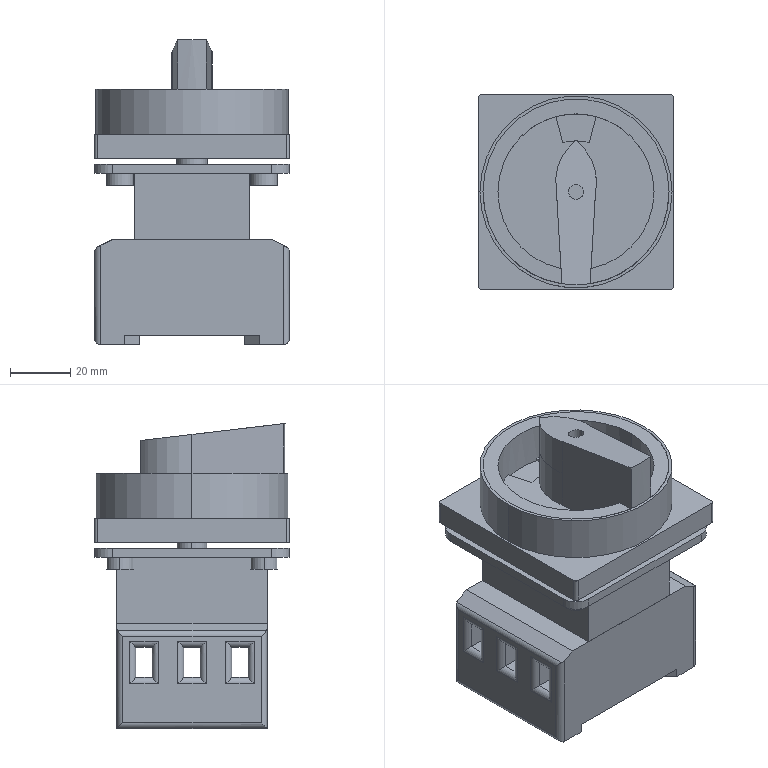Part | STEP file | Changeover switch LW30-63.... | 6 solids | 177 faces | box 65 x 65 x 101.647 mm | volume 216311 mm3 | cylinder 82 | plane 71 | cone 20 | spline 4 | commonest cylinder face diameters 4 x32 6.5 x12 3.3 x8 9 x8 2 x4 12 x4